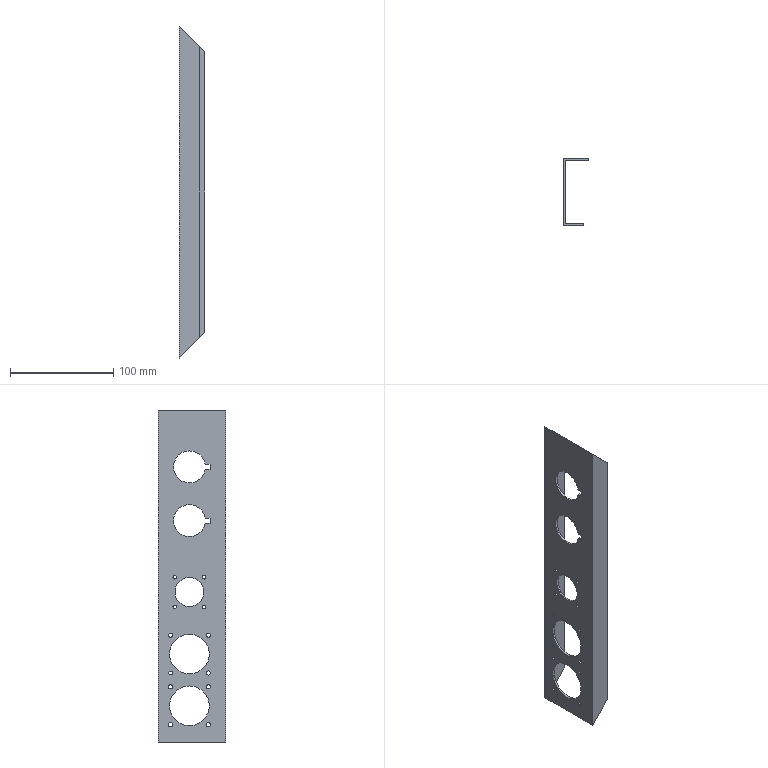Part | STEP file | 1540D1D2-2-V2.stp.STEP | 1 solid | 52 faces | box 25 x 65 x 321 mm | volume 56493 mm3 | cylinder 36 | plane 16 | commonest cylinder face diameters 4 x10 3.4 x8 3.81 x6 31 x6 38.5 x4 28 x2